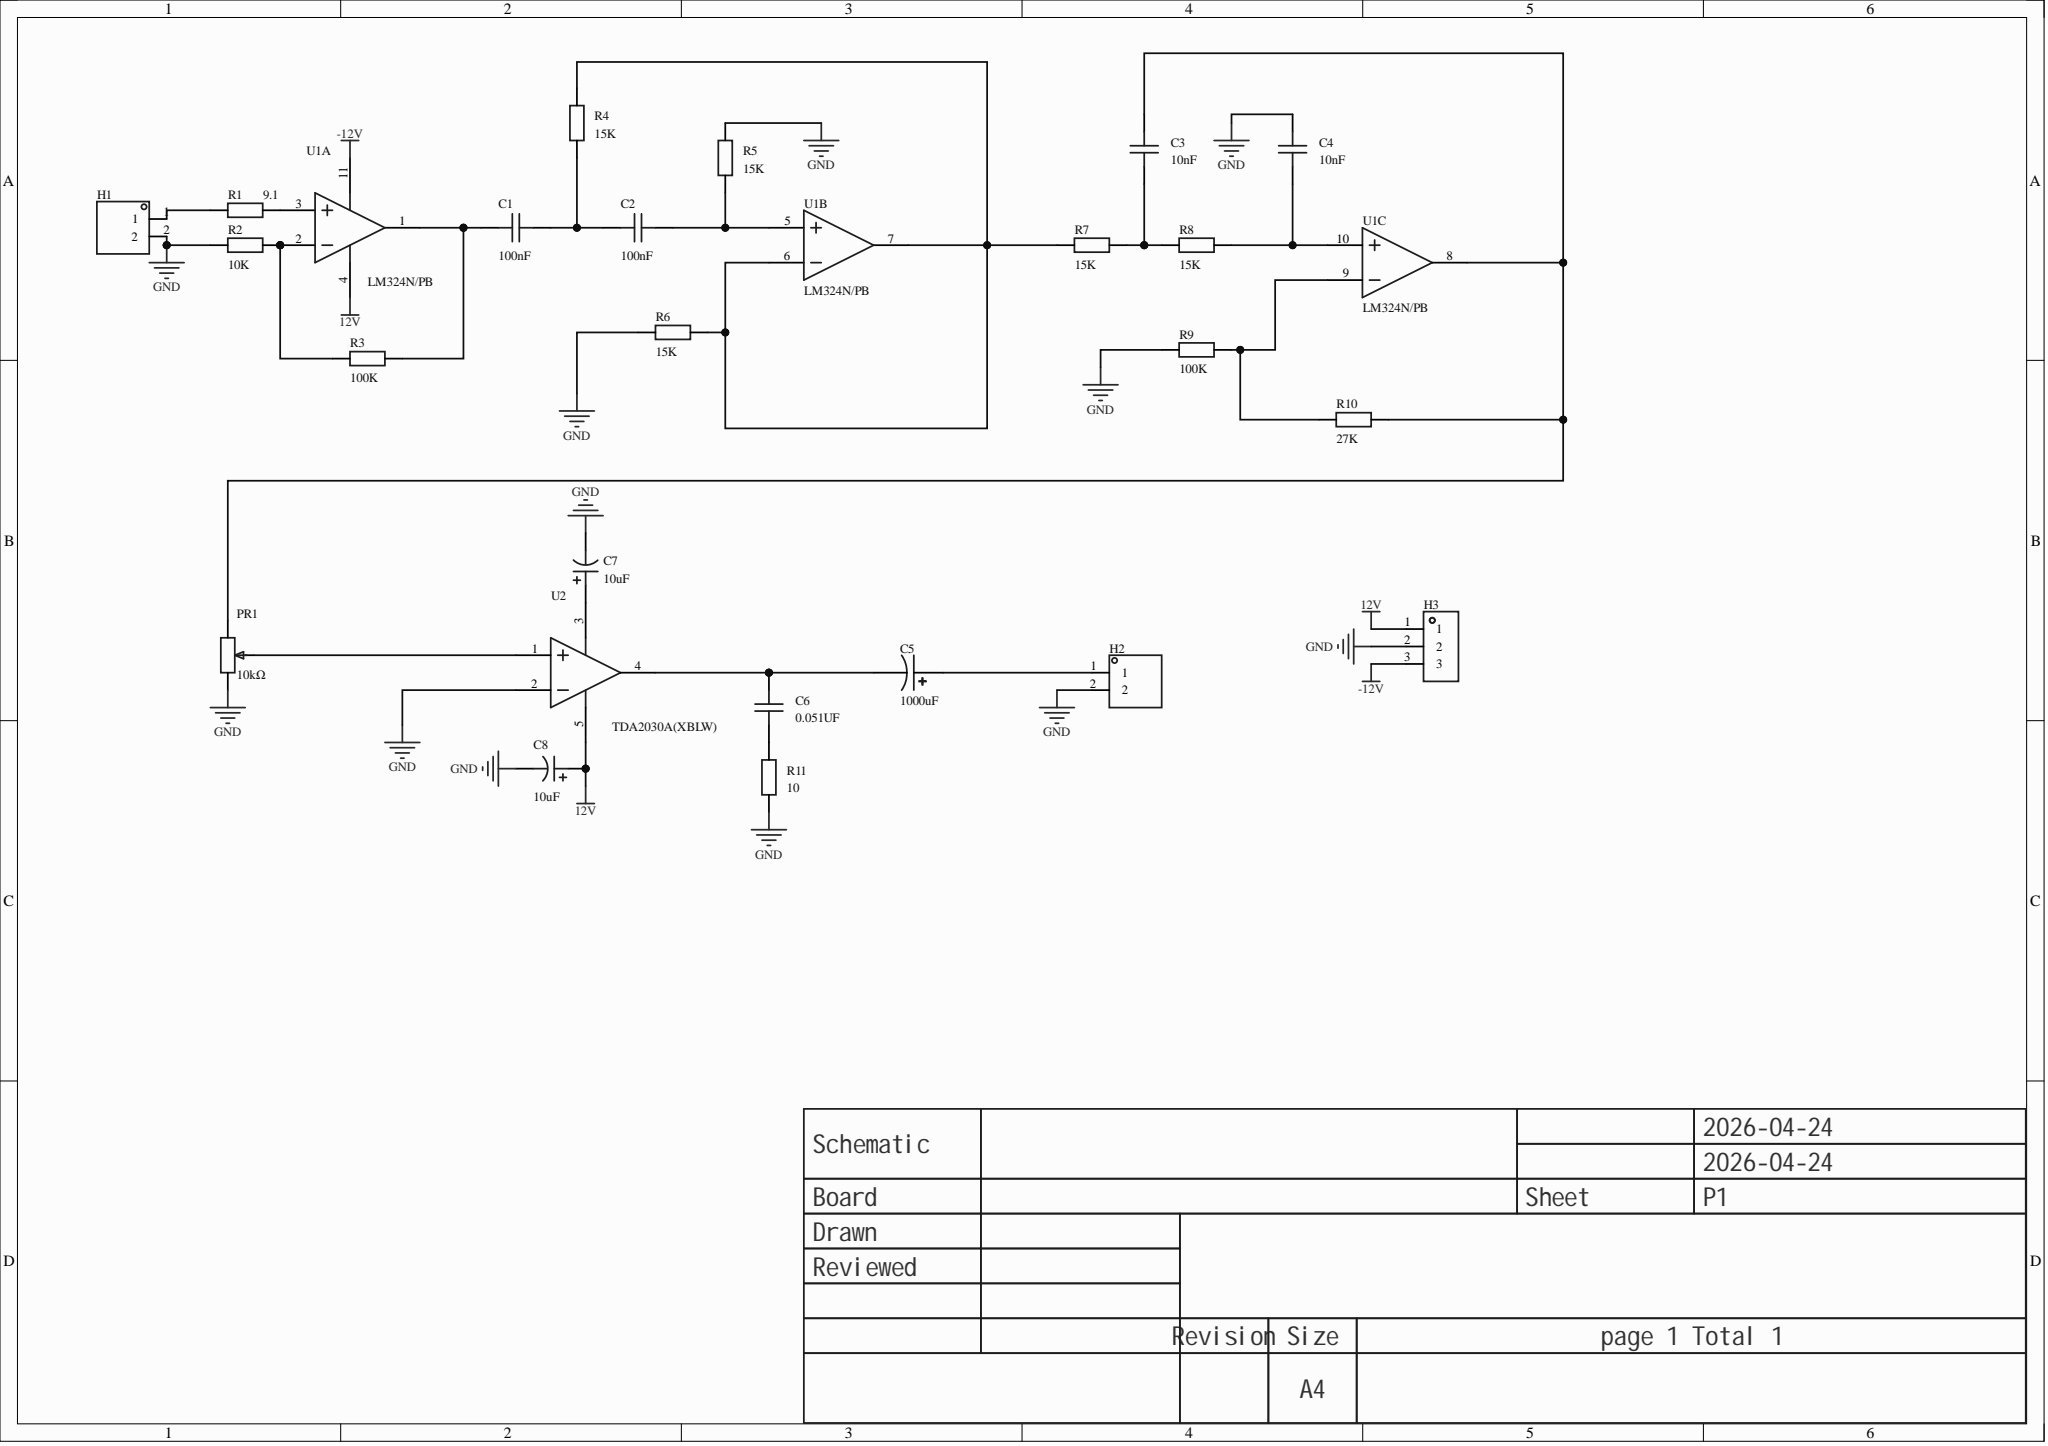Circuit board | Altium Designer | 25 parts | 19 nets
Bill of materials:
Comment,Description,Designator,Footprint,LibRef,Quantity
"100nF","","C1, C2","C0603","CAP_0603","2"
"10nF","","C3, C4","C0603","CAP_0603","2"
"1000uF","Capacitance:1000uF;Tolerance:±20%;Rated voltage:50V;Ripple current:2.286A@120Hz;Equivalent series resistance(ESR):-;","C5","CAP-TH_BD12.5-P5.00-D0.6-FD","50ZLJ1000M12.5X35","1"
"0.051UF","","C6","C0603","CAP_0603","1"
"10uF","Capacitance:10uF;Tolerance:±20%;Rated voltage:50V;Ripple current:120mA@100KHz;Equivalent series resistance(ESR):1.6Ω;","C7, C8","CAP-TH_BD5.0-P2.00-D0.8-FD-10UF50VC110GL","10UF50VC110GL","2"
"","","H1, H2","HDR-TH_2P-P2.54-V-M-1","HDR-M_2.54_1x2P","2"
"","","H3","HDR-TH_3P-P2.54-V-M","HDR-M_2.54_1x3P","1"
"10kΩ","","PR1","R_3296","R_3296","1"
"9.1","","R1","R0603","Res_0603","1"
"10K","","R2","R0603","Res_0603","1"
"100K","","R3, R9","R0603","Res_0603","2"
"15K","","R4, R5, R6, R7, R8","R0603","Res_0603","5"
"27K","","R10","R0603","Res_0603","1"
"10","","R11","R0603","Res_0603","1"
"LM324N/PB","Amplifier count:4;Rail-to-rail:-;Gain bandwidth product(GBW):-;Input offset voltage(Vos):2mV;Slew rate(SR):-;Input bias current(Ib):45nA;","U1","PDIP-14_L19.2-W6.6-P2.54-LS7.6-BL","LM324N/PB","1"
"TDA2030A(XBLW)","Amplifier type:Class AB amplifier;Speaker channels:-;Output power:25W;Quiescent current(Iq):26mA;","U2","TO-220-5_L10.5-W15.5-P1.70-TL","TDA2030A(XBLW)","1"
Netlist (Protel format):
[
C1
C0603
100nF



]
[
C2
C0603
100nF



]
[
C3
C0603
10nF



]
[
C4
C0603
10nF



]
[
C5
CAP-TH_BD12.5-P5.00-D0.6-FD
1000uF



]
[
C6
C0603
0.051UF



]
[
C7
CAP-TH_BD5.0-P2.00-D0.8-FD-10UF50VC110GL
10uF



]
[
C8
CAP-TH_BD5.0-P2.00-D0.8-FD-10UF50VC110GL
10uF



]
[
H1
HDR-TH_2P-P2.54-V-M-1




]
[
H2
HDR-TH_2P-P2.54-V-M-1




]
[
H3
HDR-TH_3P-P2.54-V-M




]
[
PR1
R_3296
10kΩ



]
[
R1
R0603
9.1



]
[
R2
R0603
10K



]
[
R3
R0603
100K



]
[
R4
R0603
15K



]
[
R5
R0603
15K



]
[
R6
R0603
15K



]
[
R7
R0603
15K



]
[
R8
R0603
15K



]
[
R9
R0603
100K



]
[
R10
R0603
27K



]
[
R11
R0603
10



]
[
U1
PDIP-14_L19.2-W6.6-P2.54-LS7.6-BL
LM324N/PB



]
[
U2
TO-220-5_L10.5-W15.5-P1.70-TL
TDA2030A(XBLW)



]
(
NetR9_2
R9-2
R10-1
U1-9
)
(
NetR4_2
R4-2
R6-1
R7-1
U1-6
U1-7
)
(
NetR2_2
R2-2
R3-1
U1-2
)
(
NetR1_2
R1-2
U1-3
)
(
NetPR1_2
PR1-2
U2-1
)
(
NetH1_1
H1-1
R1-1
)
(
NetC7_1
C7-1
U2-3
)
(
NetC6_1
C6-1
R11-2
)
(
NetC5_2
C5-2
C6-2
U2-4
)
(
NetC5_1
C5-1
H2-1
)
(
NetC4_1
C4-1
R8-2
U1-10
)
(
NetC3_2
C3-2
PR1-3
R10-2
U1-8
)
(
NetC3_1
C3-1
R7-2
R8-1
)
(
NetC2_2
C2-2
R5-1
U1-5
)
(
NetC1_2
C1-2
C2-1
R4-1
)
(
NetC1_1
C1-1
R3-2
U1-1
)
(
GND
C4-2
C7-2
C8-2
H1-2
H2-2
H3-2
PR1-1
R2-1
R5-2
R6-2
R9-1
R11-1
U2-2
)
(
-12V
H3-3
U1-11
)
(
12V
C8-1
H3-1
U1-4
U2-5
)